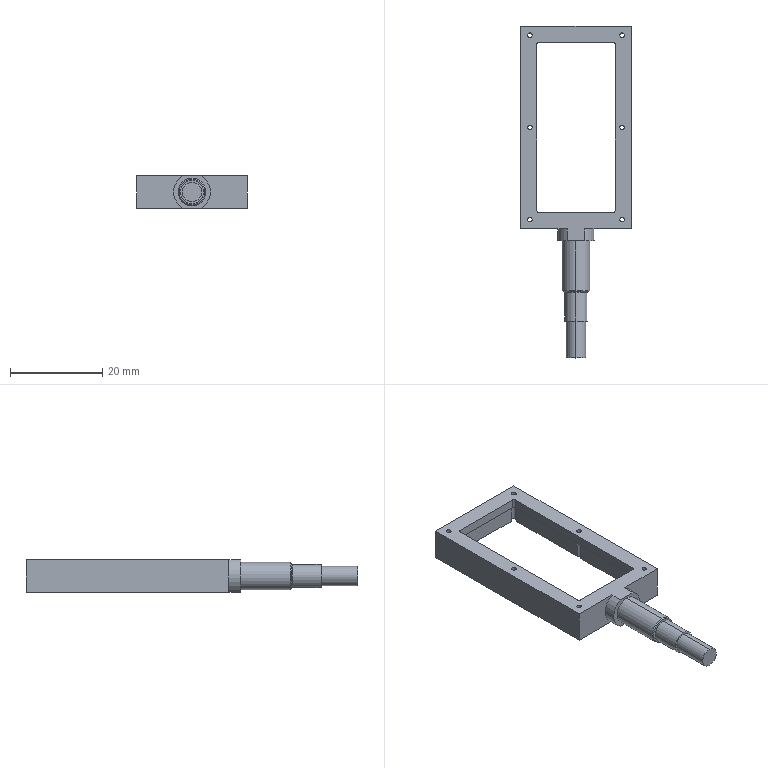NC program | NX | posted with a generic post | part box 24 x 72 x 7 mm
Lines 1 to 2080 of 5160, first 1994 of 2064 lines:
N10 G17 G21 G94 G90
(FLOOR_WALL , TOOL : D10)
N12 T10 M6
N14 G54
N16 G17 G0 G90 X-11.482 Y22. S9500 M3
N18 G43 Z30. H10
N20 Z2.505
N22 G94 G1 Z-0.495 F1000.
N24 X-3.482
N26 Y0. F2500.
N28 X3.482
N30 Y44.
N32 X-3.482
N34 Y22.
N36 X-11.482
N38 Z2.505
N40 G0 Z30.
N42 X-12.873
N44 Z2.011
N46 G1 Z-0.989 F1000.
N48 X0.373
N50 Y39.5 F2500.
N52 X-0.373
N54 Y4.5
N56 X0.373
N58 Y22.
N60 X4.873
N62 Y44.
N64 X-4.873
N66 Y0.
N68 X4.873
N70 Y22.
N72 X12.873
N74 Z2.011
N76 G0 Z30.
N78 X13.907
N80 Z1.516
N82 G1 Z-1.484 F1000.
N84 X0.907
N86 Y39. F2500.
N88 X-0.907
N90 Y5.
N92 X0.907
N94 Y22.
N96 X5.907
N98 Y44.
N100 X-5.907
N102 Y0.
N104 X5.907
N106 Y22.
N108 X13.907
N110 Z1.516
N112 G0 Z30.
N114 X14.748
N116 Z1.022
N118 G1 Z-1.978 F1000.
N120 X1.748
N122 Y39. F2500.
N124 X-1.748
N126 Y5.
N128 X1.748
N130 Y22.
N132 X6.748
N134 Y44.
N136 X-6.748
N138 Y0.
N140 X6.748
N142 Y22.
N144 X14.748
N146 Z1.022
N148 G0 Z30.
N150 X15.463
N152 Z0.528
N154 G1 Z-2.472 F1000.
N156 X2.463
N158 Y39. F2500.
N160 X-2.463
N162 Y5.
N164 X2.463
N166 Y22.
N168 X7.463
N170 Y44.
N172 X-7.463
N174 Y0.
N176 X7.463
N178 Y22.
N180 X15.463
N182 Z0.528
N184 G0 Z30.
N186 X16.085
N188 Z0.033
N190 G1 Z-2.967 F1000.
N192 X3.085
N194 Y39. F2500.
N196 X-3.085
N198 Y5.
N200 X3.085
N202 Y22.
N204 X8.085
N206 Y44.
N208 X-8.085
N210 Y0.
N212 X8.085
N214 Y22.
N216 X16.085
N218 Z0.033
N220 G0 Z30.
N222 X16.634
N224 Z-0.461
N226 G1 Z-3.461 F1000.
N228 X3.634
N230 Y39. F2500.
N232 X-3.634
N234 Y5.
N236 X3.634
N238 Y22.
N240 X8.634
N242 Y44.
N244 X-8.634
N246 Y0.
N248 X8.634
N250 Y22.
N252 X16.634
N254 Z-0.461
N256 G0 Z30.
N258 X17.124
N260 Z-0.956
N262 G1 Z-3.956 F1000.
N264 X4.124
N266 Y39. F2500.
N268 X-4.124
N270 Y5.
N272 X4.124
N274 Y22.
N276 X9.124
N278 Y44.
N280 X-9.124
N282 Y0.
N284 X9.124
N286 Y22.
N288 X17.124
N290 Z-0.956
N292 G0 Z30.
N294 X-0.063 Y9.915
N296 Z-0.956
N298 G1 Y9.5 Z-1.067 F1000.
N300 X0.063 Z-1.101
N302 Y22. Z-4.45
N304 Y34.5 F2500.
N306 X-0.063
N308 Y9.5
N310 X0.063
N312 Y22.
N314 X4.563
N316 Y39.
N318 X-4.563
N320 Y5.
N322 X4.563
N324 Y22.
N326 X9.563
N328 Y44.
N330 X-9.563
N332 Y0.
N334 X9.563
N336 Y22.
N338 X17.563
N340 Z-1.45
N342 G0 Z30.
N344 X-0.083 Y9.5
N346 Z-1.45
N348 G1 X0.458 Z-1.595 F1000.
N350 Y22. Z-4.945
N352 Y34.5 F2500.
N354 X-0.458
N356 Y9.5
N358 X0.458
N360 Y22.
N362 X4.958
N364 Y39.
N366 X-4.958
N368 Y5.
N370 X4.958
N372 Y22.
N374 X9.958
N376 Y44.
N378 X-9.958
N380 Y0.
N382 X9.958
N384 Y22.
N386 X17.958
N388 Z-1.945
N390 G0 Z30.
N392 X0.315 Y33.588
N394 Z-1.945
N396 G1 Y34. Z-2.055 F1000.
N398 X-0.315 Z-2.224
N400 Y22. Z-5.439
N402 Y10. F2500.
N404 X0.315
N406 Y34.
N408 X-0.315
N410 Y22.
N412 X-5.315
N414 Y5.
N416 X5.315
N418 Y39.
N420 X-5.315
N422 Y22.
N424 X-10.315
N426 Y0.
N428 X10.315
N430 Y44.
N432 X-10.315
N434 Y22.
N436 X-18.315
N438 Z-2.439
N440 G0 Z30.
N442 X0.405 Y34.
N444 Z-2.439
N446 G1 X-0.636 Z-2.718 F1000.
N448 Y22. Z-5.933
N450 Y10. F2500.
N452 X0.636
N454 Y34.
N456 X-0.636
N458 Y22.
N460 X-5.636
N462 Y5.
N464 X5.636
N466 Y39.
N468 X-5.636
N470 Y22.
N472 X-10.636
N474 Y0.
N476 X10.636
N478 Y44.
N480 X-10.636
N482 Y22.
N484 X-18.636
N486 Z-2.933
N488 G0 Z30.
N490 X-0.115 Y10.
N492 Z-2.933
N494 G1 X0.926 Z-3.212 F1000.
N496 Y22. Z-6.428
N498 Y34. F2500.
N500 X-0.926
N502 Y10.
N504 X0.926
N506 Y22.
N508 X5.926
N510 Y39.
N512 X-5.926
N514 Y5.
N516 X5.926
N518 Y22.
N520 X10.926
N522 Y44.
N524 X-10.926
N526 Y0.
N528 X10.926
N530 Y22.
N532 X18.926
N534 Z-3.428
N536 G0 Z30.
N538 X-0.145 Y34.
N540 Z-3.428
N542 G1 X-1.187 Z-3.707 F1000.
N544 Y22. Z-6.922
N546 Y10. F2500.
N548 X1.187
N550 Y34.
N552 X-1.187
N554 Y22.
N556 X-6.187
N558 Y5.
N560 X6.187
N562 Y39.
N564 X-6.187
N566 Y22.
N568 X-11.187
N570 Y0.
N572 X11.187
N574 Y44.
N576 X-11.187
N578 Y22.
N580 X-19.187
N582 Z-3.922
N584 G0 Z30.
N586 X-0.378 Y34.
N588 Z-3.922
N590 G1 X-1.42 Z-4.201 F1000.
N592 Y22. Z-7.417
N594 Y10. F2500.
N596 X1.42
N598 Y34.
N600 X-1.42
N602 Y22.
N604 X-6.42
N606 Y5.
N608 X6.42
N610 Y39.
N612 X-6.42
N614 Y22.
N616 X-11.42
N618 Y0.
N620 X11.42
N622 Y44.
N624 X-11.42
N626 Y22.
N628 X-19.42
N630 Z-4.417
N632 G0 Z30.
N634 X0.586 Y10.
N636 Z-4.417
N638 G1 X1.627 Z-4.696 F1000.
N640 Y22. Z-7.911
N642 Y34. F2500.
N644 X-1.627
N646 Y10.
N648 X1.627
N650 Y22.
N652 X6.627
N654 Y39.
N656 X-6.627
N658 Y5.
N660 X6.627
N662 Y22.
N664 X11.627
N666 Y44.
N668 X-11.627
N670 Y0.
N672 X11.627
N674 Y22.
N676 X19.627
N678 Z-4.911
N680 G0 Z30.
N682 X0.769 Y10.
N684 Z-4.911
N686 G1 X1.81 Z-5.19 F1000.
N688 Y22. Z-8.406
N690 Y34. F2500.
N692 X-1.81
N694 Y10.
N696 X1.81
N698 Y22.
N700 X6.81
N702 Y39.
N704 X-6.81
N706 Y5.
N708 X6.81
N710 Y22.
N712 X11.81
N714 Y44.
N716 X-11.81
N718 Y0.
N720 X11.81
N722 Y22.
N724 X19.81
N726 Z-5.406
N728 G0 Z30.
N730 X-0.929 Y34.003
N732 Z-5.406
N734 G1 X-1.97 Y34. Z-5.685 F1000.
N736 Y22. Z-8.9
N738 Y10. F2500.
N740 X1.97
N742 Y34.
N744 X1.744
N746 G2 X0. Y34.153 R10.
N748 X-1.744 Y34. R10.
N750 G1 X-1.97
N752 Y22.
N754 X-6.97
N756 Y5.
N758 X6.97
N760 Y39.
N762 X1.744
N764 G2 X0. Y39.314 R5.
N766 X-1.744 Y39. R5.
N768 G1 X-6.97
N770 Y22.
N772 X-11.97
N774 Y0.
N776 X11.97
N778 Y44.
N780 X1.744
N782 Y46.6
N784 X-1.744
N786 Y44.
N788 X-11.97
N790 Y22.
N792 X-19.97
N794 Z-5.9
N796 G0 Z30.
N798 M5
(DRILLING_COPY_1 , TOOL : D6A45)
N800 T07 M6
N802 G54
N804 G17 G0 G90 X-10. Y2. S5000 M3
N806 G43 Z30. H7
N808 G94 G81 G98 Z-10. F250. R-6.
N810 X-11. Y9.
N812 X-10. Y22.
N814 X-11. Y35.
N816 X-10. Y42.
N818 X10.
N820 X11. Y35.
N822 X10. Y22.
N824 X11. Y9.
N826 X10. Y2.
N828 G80
N830 G0 X10. Y2. Z30.
N832 M5
(DRILLING_COPY , TOOL : 1.25ZT)
N834 T14 M6
N836 G54
N838 G17 G0 G90 X11. Y35. S2009 M3
N840 G43 Z30. H14
N842 G94 G83 G98 Z-13.626 F100. Q2. R-6.
N844 X-11.
N846 Y9.
N848 X11.
N850 G80
N852 G0 X11. Y9. Z30.
N854 M5
(DRILLING_COPY_COPY , TOOL : 1.0ZT)
N856 T13 M6
N858 G54
N860 G17 G0 G90 X-10. Y22. S2009 M3
N862 G43 Z30. H13
N864 G94 G83 G98 Z-16.8 F100. Q2. R-6.
N866 Y2.
N868 X10.
N870 Y22.
N872 Y42.
N874 X-10.
N876 G80
N878 G0 X-10. Y42. Z30.
N880 M5
(CAVITY_MILL , TOOL : D10)
N882 T10 M6
N884 G54
N886 G17 G0 G90 X-19.132 Y24.145 S9500 M3
N888 G43 Z30. H10
N890 Z-8.49
N892 G94 G1 Z-9.49 F1000.
N894 X-17.489 Y22.766
N896 G2 X-17.132 Y22. R1.
N898 G1 Y0. F2500.
N900 G3 X-17. Y-1.143 R4.999
N902 G1 Y-1.005
N904 G2 X-17.1 Y0. R5.1
N906 G1 Y44.
N908 G2 X-17. Y45.005 R5.1
N910 G1 Y45.143
N912 G3 X-17.132 Y44. R4.999
N914 G1 Y22.
N916 G2 X-17.489 Y21.234 R1.
N918 G1 X-19.132 Y19.855
N920 Z-8.49
N922 G0 X-19.243 Y24.145 Z-8.98
N924 G1 Z-9.98 F1000.
N926 X-17.601 Y22.766
N928 G2 X-17.243 Y22. R1.
N930 G1 X-17.1
N932 Y44. F2500.
N934 G2 X-17. Y45.005 R5.1
N936 G1 Y45.541
N938 G3 X-17.243 Y44. R4.999
N940 G1 Y0.
N942 G3 X-17. Y-1.541 R4.999
N944 G1 Y-1.005
N946 G2 X-17.1 Y0. R5.1
N948 G1 Y22.
N950 G3 X-17.457 Y22.766 R1.
N952 G1 X-19.243 Y24.265
N954 Z-8.98
N956 G0 X-19.334 Y24.145 Z-9.47
N958 G1 Z-10.47 F1000.
N960 X-17.691 Y22.766
N962 G2 X-17.334 Y22. R1.
N964 G1 X-17.1
N966 Y44. F2500.
N968 G2 X-17. Y45.005 R5.1
N970 G1 Y45.797
N972 G3 X-17.334 Y44. R5.
N974 G1 Y0.
N976 G3 X-17. Y-1.797 R5.
N978 G1 Y-1.005
N980 G2 X-17.1 Y0. R5.1
N982 G1 Y22.
N984 G3 X-17.457 Y22.766 R1.
N986 G1 X-19.334 Y24.341
N988 Z-9.47
N990 G0 X-19.405 Y24.145 Z-9.96
N992 G1 Z-10.96 F1000.
N994 X-17.762 Y22.766
N996 G2 X-17.405 Y22. R1.
N998 G1 X-17.1
N1000 Y44. F2500.
N1002 G2 X-17. Y45.005 R5.1
N1004 G1 Y45.955
N1006 G3 X-17.405 Y44. R5.021
N1008 G1 Y0.
N1010 G3 X-17. Y-1.971 R5.
N1012 G1 Y-1.005
N1014 G2 X-17.1 Y0. R5.1
N1016 G1 Y22.
N1018 G3 X-17.457 Y22.766 R1.
N1020 G1 X-19.405 Y24.4
N1022 Z-9.96
N1024 G0 X-19.456 Y24.145 Z-10.45
N1026 G1 Z-11.45 F1000.
N1028 X-17.813 Y22.766
N1030 G2 X-17.456 Y22. R1.
N1032 G1 X-17.1
N1034 Y44. F2500.
N1036 G2 X-17. Y45.005 R5.1
N1038 G1 Y46.065
N1040 G3 X-17.456 Y44. R5.028
N1042 G1 Y0.
N1044 G3 X-17. Y-2.065 R5.027
N1046 G1 Y-1.005
N1048 G2 X-17.1 Y0. R5.1
N1050 G1 Y22.
N1052 G3 X-17.457 Y22.766 R1.
N1054 G1 X-19.456 Y24.443
N1056 Z-10.45
N1058 G0 X-19.487 Y24.145 Z-10.94
N1060 G1 Z-11.94 F1000.
N1062 X-17.845 Y22.766
N1064 G2 X-17.487 Y22. R1.
N1066 G1 X-17.1
N1068 Y44. F2500.
N1070 G2 X-17. Y45.005 R5.1
N1072 G1 Y46.14
N1074 G3 X-17.487 Y44. R5.018
N1076 G1 Y0.034
N1078 G3 X-17. Y-2.14 R5.017
N1080 G1 Y-1.005
N1082 G2 X-17.1 Y0. R5.1
N1084 G1 Y22.
N1086 G3 X-17.457 Y22.766 R1.
N1088 G1 X-19.487 Y24.47
N1090 Z-10.94
N1092 G0 X-19.5 Y24.145 Z-11.43
N1094 G1 Z-12.43 F1000.
N1096 X-17.857 Y22.766
N1098 G2 X-17.5 Y22. R1.
N1100 G1 X-17.1
N1102 Y44. F2500.
N1104 G2 X-17. Y45.005 R5.1
N1106 G1 Y46.179
N1108 G3 X-17.5 Y44. R5.001
N1110 G1 Y0.
N1112 G3 X-17. Y-2.176 R5.004
N1114 G1 Y-1.005
N1116 G2 X-17.1 Y0. R5.1
N1118 G1 Y22.
N1120 G3 X-17.457 Y22.766 R1.
N1122 G1 X-19.5 Y24.48
N1124 Z-11.43
N1126 G0 Y24.144 Z-11.92
N1128 G1 Z-12.92 F1000.
N1130 X-17.857 Y22.766
N1132 G2 X-17.5 Y22. R1.
N1134 G1 X-17.35
N1136 X-17.1
N1138 Y44. F2500.
N1140 G2 X-17. Y45.005 R5.1
N1142 G1 Y46.179
N1144 G3 X-17.5 Y44.011 R5.
N1146 G1 X-17.499 Y0.
N1148 G3 X-17. Y-2.173 R5.007
N1150 G1 Y-1.005
N1152 G2 X-17.1 Y0. R5.1
N1154 G1 Y22.
N1156 G3 X-17.457 Y22.766 R1.
N1158 G1 X-19.5 Y24.48
N1160 Z-11.92
N1162 G0 Y24.144 Z-12.41
N1164 G1 Z-13.41 F1000.
N1166 X-17.857 Y22.766
N1168 G2 X-17.5 Y22. R1.
N1170 G1 X-17.35
N1172 X-17.1
N1174 Y44. F2500.
N1176 G2 X-17. Y45.005 R5.1
N1178 G1 Y46.179
N1180 G3 X-17.5 Y44.011 R5.
N1182 G1 X-17.499 Y0.
N1184 G3 X-17. Y-2.173 R5.007
N1186 G1 Y-1.005
N1188 G2 X-17.1 Y0. R5.1
N1190 G1 Y22.
N1192 G3 X-17.457 Y22.766 R1.
N1194 G1 X-19.5 Y24.48
N1196 Z-12.41
N1198 G0 Y24.144 Z-12.9
N1200 G1 Z-13.9 F1000.
N1202 X-17.857 Y22.766
N1204 G2 X-17.5 Y22. R1.
N1206 G1 X-17.35
N1208 X-17.1
N1210 Y44. F2500.
N1212 G2 X-17. Y45.005 R5.1
N1214 G1 Y46.179
N1216 G3 X-17.5 Y44.011 R5.
N1218 G1 X-17.499 Y0.
N1220 G3 X-17. Y-2.173 R5.007
N1222 G1 Y-1.005
N1224 G2 X-17.1 Y0. R5.1
N1226 G1 Y22.
N1228 G3 X-17.457 Y22.766 R1.
N1230 G1 X-19.5 Y24.48
N1232 Z-12.9
N1234 G0 Y24.144 Z-13.32
N1236 G1 Z-14.32 F1000.
N1238 X-17.857 Y22.766
N1240 G2 X-17.5 Y22. R1.
N1242 G1 X-17.35
N1244 X-17.1
N1246 Y44. F2500.
N1248 G2 X-17. Y45.005 R5.1
N1250 G1 Y46.179
N1252 G3 X-17.5 Y44.011 R5.
N1254 G1 X-17.499 Y0.
N1256 G3 X-17. Y-2.173 R5.007
N1258 G1 Y-1.005
N1260 G2 X-17.1 Y0. R5.1
N1262 G1 Y22.
N1264 G3 X-17.457 Y22.766 R1.
N1266 G1 X-19.5 Y24.48
N1268 Z-13.32
N1270 G0 Y24.144 Z-13.74
N1272 G1 Z-14.74 F1000.
N1274 X-17.857 Y22.766
N1276 G2 X-17.5 Y22. R1.
N1278 G1 X-17.35
N1280 X-17.1
N1282 Y44. F2500.
N1284 G2 X-17. Y45.005 R5.1
N1286 G1 Y46.179
N1288 G3 X-17.5 Y44.011 R5.
N1290 G1 X-17.499 Y0.
N1292 G3 X-17. Y-2.173 R5.007
N1294 G1 Y-1.005
N1296 G2 X-17.1 Y0. R5.1
N1298 G1 Y22.
N1300 G3 X-17.457 Y22.766 R1.
N1302 G1 X-19.5 Y24.48
N1304 Z-13.74
N1306 G0 Y24.144 Z-14.16
N1308 G1 Z-15.16 F1000.
N1310 X-17.857 Y22.766
N1312 G2 X-17.5 Y22. R1.
N1314 G1 X-17.35
N1316 X-17.1
N1318 Y44. F2500.
N1320 G2 X-17. Y45.005 R5.1
N1322 G1 Y46.179
N1324 G3 X-17.5 Y44.011 R5.
N1326 G1 Y0.005
N1328 G3 X-17. Y-2.173 R5.008
N1330 G1 Y-1.005
N1332 G2 X-17.1 Y0. R5.1
N1334 G1 Y22.
N1336 G3 X-17.457 Y22.766 R1.
N1338 G1 X-19.5 Y24.48
N1340 Z-14.16
N1342 G0 Y24.144 Z-14.58
N1344 G1 Z-15.58 F1000.
N1346 X-17.857 Y22.766
N1348 G2 X-17.5 Y22. R1.
N1350 G1 X-17.35
N1352 X-17.1
N1354 Y44. F2500.
N1356 G2 X-17. Y45.005 R5.1
N1358 G1 Y46.179
N1360 G3 X-17.5 Y44.011 R5.
N1362 G1 Y0.005
N1364 G3 X-17. Y-2.173 R5.008
N1366 G1 Y-1.005
N1368 G2 X-17.1 Y0. R5.1
N1370 G1 Y22.
N1372 G3 X-17.457 Y22.766 R1.
N1374 G1 X-19.5 Y24.48
N1376 Z-14.58
N1378 G0 Y24.144 Z-15.
N1380 G1 Z-16. F1000.
N1382 X-17.857 Y22.766
N1384 G2 X-17.5 Y22. R1.
N1386 G1 X-17.35
N1388 X-17.1
N1390 Y44. F2500.
N1392 G2 X-17. Y45.005 R5.1
N1394 G1 Y46.179
N1396 G3 X-17.5 Y44.011 R5.
N1398 G1 Y0.005
N1400 G3 X-17. Y-2.173 R5.008
N1402 G1 Y-1.005
N1404 G2 X-17.1 Y0. R5.1
N1406 G1 Y22.
N1408 G3 X-17.457 Y22.766 R1.
N1410 G1 X-19.5 Y24.48
N1412 Z-15.
N1414 G0 Z30.
N1416 X-0.4 Y16.77
N1418 Z-7.5
N1420 G1 Y11.6 Z-7.771 F1000.
N1422 X0.4 Z-7.813
N1424 Y21.75 Z-8.345
N1426 X0.413 Y22. Z-8.358
N1428 X0.4 Y22.25 Z-8.371
N1430 Y32.4 Z-8.903
N1432 X-0.4 Z-8.945
N1434 Y22.25 Z-9.477
N1436 X-0.413 Y22. Z-9.49
N1438 G2 X-0.4 Y21.5 R9.6 F2500.
N1440 G1 Y11.6
N1442 X0.4
N1444 Y21.5
N1446 G2 X0.413 Y22. R9.6
N1448 X0.4 Y22.5 R9.6
N1450 G1 Y32.4
N1452 X-0.4
N1454 Y22.5
N1456 G2 X-0.413 Y22. R9.6
N1458 G1 X-4.907 Y22.234
N1460 G2 X-4.925 Y22. R5.1
N1462 X-4.9 Y21.5 R5.1
N1464 G1 Y7.1
N1466 X4.9
N1468 Y21.5
N1470 G2 X4.925 Y22. R5.1
N1472 X4.9 Y22.5 R5.1
N1474 G1 Y36.9
N1476 X-4.9
N1478 Y22.5
N1480 G2 X-4.907 Y22.234 R5.1
N1482 G3 X-4.59 Y21.451 R1.
N1484 G1 Z-8.49
N1486 G0 Z30.
N1488 X-0.4 Y16.77
N1490 Z-7.99
N1492 G1 Y11.6 Z-8.261 F1000.
N1494 X0.4 Z-8.303
N1496 Y21.75 Z-8.835
N1498 X0.413 Y22. Z-8.848
N1500 X0.4 Y22.25 Z-8.861
N1502 Y32.4 Z-9.393
N1504 X-0.4 Z-9.435
N1506 Y22.25 Z-9.967
N1508 X-0.413 Y22. Z-9.98
N1510 G2 X-0.4 Y21.5 R9.6 F2500.
N1512 G1 Y11.6
N1514 X0.4
N1516 Y21.5
N1518 G2 X0.413 Y22. R9.6
N1520 X0.4 Y22.5 R9.6
N1522 G1 Y32.4
N1524 X-0.4
N1526 Y22.5
N1528 G2 X-0.413 Y22. R9.6
N1530 G1 X-4.907 Y22.234
N1532 G2 X-4.925 Y22. R5.1
N1534 X-4.9 Y21.5 R5.1
N1536 G1 Y7.1
N1538 X4.9
N1540 Y21.5
N1542 G2 X4.925 Y22. R5.1
N1544 X4.9 Y22.5 R5.1
N1546 G1 Y36.9
N1548 X-4.9
N1550 Y22.5
N1552 G2 X-4.907 Y22.234 R5.1
N1554 G3 X-4.59 Y21.451 R1.
N1556 G1 Z-8.98
N1558 G0 Z30.
N1560 X-0.4 Y16.77
N1562 Z-8.48
N1564 G1 Y11.6 Z-8.751 F1000.
N1566 X0.4 Z-8.793
N1568 Y21.75 Z-9.325
N1570 X0.413 Y22. Z-9.338
N1572 X0.4 Y22.25 Z-9.351
N1574 Y32.4 Z-9.883
N1576 X-0.4 Z-9.925
N1578 Y22.25 Z-10.457
N1580 X-0.413 Y22. Z-10.47
N1582 G2 X-0.4 Y21.5 R9.6 F2500.
N1584 G1 Y11.6
N1586 X0.4
N1588 Y21.5
N1590 G2 X0.413 Y22. R9.6
N1592 X0.4 Y22.5 R9.6
N1594 G1 Y32.4
N1596 X-0.4
N1598 Y22.5
N1600 G2 X-0.413 Y22. R9.6
N1602 G1 X-4.907 Y22.234
N1604 G2 X-4.925 Y22. R5.1
N1606 X-4.9 Y21.5 R5.1
N1608 G1 Y7.1
N1610 X4.9
N1612 Y21.5
N1614 G2 X4.925 Y22. R5.1
N1616 X4.9 Y22.5 R5.1
N1618 G1 Y36.9
N1620 X-4.9
N1622 Y22.5
N1624 G2 X-4.907 Y22.234 R5.1
N1626 G3 X-4.59 Y21.451 R1.
N1628 G1 Z-9.47
N1630 G0 X-0.4 Y16.77 Z-8.97
N1632 G1 Y11.6 Z-9.241 F1000.
N1634 X0.4 Z-9.283
N1636 Y21.75 Z-9.815
N1638 X0.413 Y22. Z-9.828
N1640 X0.4 Y22.25 Z-9.841
N1642 Y32.4 Z-10.373
N1644 X-0.4 Z-10.415
N1646 Y22.25 Z-10.947
N1648 X-0.413 Y22. Z-10.96
N1650 G2 X-0.4 Y21.5 R9.6 F2500.
N1652 G1 Y11.6
N1654 X0.4
N1656 Y21.5
N1658 G2 X0.413 Y22. R9.6
N1660 X0.4 Y22.5 R9.6
N1662 G1 Y32.4
N1664 X-0.4
N1666 Y22.5
N1668 G2 X-0.413 Y22. R9.6
N1670 G1 X-4.907 Y22.234
N1672 G2 X-4.925 Y22. R5.1
N1674 X-4.9 Y21.5 R5.1
N1676 G1 Y7.1
N1678 X4.9
N1680 Y21.5
N1682 G2 X4.925 Y22. R5.1
N1684 X4.9 Y22.5 R5.1
N1686 G1 Y36.9
N1688 X-4.9
N1690 Y22.5
N1692 G2 X-4.907 Y22.234 R5.1
N1694 G3 X-4.59 Y21.451 R1.
N1696 G1 Z-9.96
N1698 G0 X-0.4 Y16.77 Z-9.46
N1700 G1 Y11.6 Z-9.731 F1000.
N1702 X0.4 Z-9.773
N1704 Y21.75 Z-10.305
N1706 X0.413 Y22. Z-10.318
N1708 X0.4 Y22.25 Z-10.331
N1710 Y32.4 Z-10.863
N1712 X-0.4 Z-10.905
N1714 Y22.25 Z-11.437
N1716 X-0.413 Y22. Z-11.45
N1718 G2 X-0.4 Y21.5 R9.6 F2500.
N1720 G1 Y11.6
N1722 X0.4
N1724 Y21.5
N1726 G2 X0.413 Y22. R9.6
N1728 X0.4 Y22.5 R9.6
N1730 G1 Y32.4
N1732 X-0.4
N1734 Y22.5
N1736 G2 X-0.413 Y22. R9.6
N1738 G1 X-4.907 Y22.234
N1740 G2 X-4.925 Y22. R5.1
N1742 X-4.9 Y21.5 R5.1
N1744 G1 Y7.1
N1746 X4.9
N1748 Y21.5
N1750 G2 X4.925 Y22. R5.1
N1752 X4.9 Y22.5 R5.1
N1754 G1 Y36.9
N1756 X-4.9
N1758 Y22.5
N1760 G2 X-4.907 Y22.234 R5.1
N1762 G3 X-4.59 Y21.451 R1.
N1764 G1 Z-10.45
N1766 G0 X-0.4 Y16.77 Z-9.95
N1768 G1 Y11.6 Z-10.221 F1000.
N1770 X0.4 Z-10.263
N1772 Y21.75 Z-10.795
N1774 X0.413 Y22. Z-10.808
N1776 X0.4 Y22.25 Z-10.821
N1778 Y32.4 Z-11.353
N1780 X-0.4 Z-11.395
N1782 Y22.25 Z-11.927
N1784 X-0.413 Y22. Z-11.94
N1786 G2 X-0.4 Y21.5 R9.6 F2500.
N1788 G1 Y11.6
N1790 X0.4
N1792 Y21.5
N1794 G2 X0.413 Y22. R9.6
N1796 X0.4 Y22.5 R9.6
N1798 G1 Y32.4
N1800 X-0.4
N1802 Y22.5
N1804 G2 X-0.413 Y22. R9.6
N1806 G1 X-4.907 Y22.234
N1808 G2 X-4.925 Y22. R5.1
N1810 X-4.9 Y21.5 R5.1
N1812 G1 Y7.1
N1814 X4.9
N1816 Y21.5
N1818 G2 X4.925 Y22. R5.1
N1820 X4.9 Y22.5 R5.1
N1822 G1 Y36.9
N1824 X-4.9
N1826 Y22.5
N1828 G2 X-4.907 Y22.234 R5.1
N1830 G3 X-4.59 Y21.451 R1.
N1832 G1 Z-10.94
N1834 G0 X-0.4 Y16.77 Z-10.44
N1836 G1 Y11.6 Z-10.711 F1000.
N1838 X0.4 Z-10.753
N1840 Y21.75 Z-11.285
N1842 X0.413 Y22. Z-11.298
N1844 X0.4 Y22.25 Z-11.311
N1846 Y32.4 Z-11.843
N1848 X-0.4 Z-11.885
N1850 Y22.25 Z-12.417
N1852 X-0.413 Y22. Z-12.43
N1854 G2 X-0.4 Y21.5 R9.6 F2500.
N1856 G1 Y11.6
N1858 X0.4
N1860 Y21.5
N1862 G2 X0.413 Y22. R9.6
N1864 X0.4 Y22.5 R9.6
N1866 G1 Y32.4
N1868 X-0.4
N1870 Y22.5
N1872 G2 X-0.413 Y22. R9.6
N1874 G1 X-4.907 Y22.234
N1876 G2 X-4.925 Y22. R5.1
N1878 X-4.9 Y21.5 R5.1
N1880 G1 Y7.1
N1882 X4.9
N1884 Y21.5
N1886 G2 X4.925 Y22. R5.1
N1888 X4.9 Y22.5 R5.1
N1890 G1 Y36.9
N1892 X-4.9
N1894 Y22.5
N1896 G2 X-4.907 Y22.234 R5.1
N1898 G3 X-4.59 Y21.451 R1.
N1900 G1 Z-11.43
N1902 G0 X-0.4 Y16.77 Z-10.93
N1904 G1 Y11.6 Z-11.201 F1000.
N1906 X0.4 Z-11.243
N1908 Y21.75 Z-11.775
N1910 X0.413 Y22. Z-11.788
N1912 X0.4 Y22.25 Z-11.801
N1914 Y32.4 Z-12.333
N1916 X-0.4 Z-12.375
N1918 Y22.25 Z-12.907
N1920 X-0.413 Y22. Z-12.92
N1922 G2 X-0.4 Y21.5 R9.6 F2500.
N1924 G1 Y11.6
N1926 X0.4
N1928 Y21.5
N1930 G2 X0.413 Y22. R9.6
N1932 X0.4 Y22.5 R9.6
N1934 G1 Y32.4
N1936 X-0.4
N1938 Y22.5
N1940 G2 X-0.413 Y22. R9.6
N1942 G1 X-4.907 Y22.234
N1944 G2 X-4.925 Y22. R5.1
N1946 X-4.9 Y21.5 R5.1
N1948 G1 Y7.1
N1950 X4.9
N1952 Y21.5
N1954 G2 X4.925 Y22. R5.1
N1956 X4.9 Y22.5 R5.1
N1958 G1 Y36.9
N1960 X-4.9
N1962 Y22.5
N1964 G2 X-4.907 Y22.234 R5.1
N1966 G3 X-4.59 Y21.451 R1.
N1968 G1 Z-11.92
N1970 G0 X-0.4 Y16.77 Z-11.42
N1972 G1 Y11.6 Z-11.691 F1000.
N1974 X0.4 Z-11.733
N1976 Y21.75 Z-12.265
N1978 X0.413 Y22. Z-12.278
N1980 X0.4 Y22.25 Z-12.291
N1982 Y32.4 Z-12.823
N1984 X-0.4 Z-12.865
N1986 Y22.25 Z-13.397
N1988 X-0.413 Y22. Z-13.41
N1990 G2 X-0.4 Y21.5 R9.6 F2500.
N1992 G1 Y11.6
N1994 X0.4
N1996 Y21.5
N1998 G2 X0.413 Y22. R9.6
N2000 X0.4 Y22.5 R9.6
N2002 G1 Y32.4
N2004 X-0.4
N2006 Y22.5
N2008 G2 X-0.413 Y22. R9.6
N2010 G1 X-4.907 Y22.234
N2012 G2 X-4.925 Y22. R5.1
N2014 X-4.9 Y21.5 R5.1
N2016 G1 Y7.1
N2018 X4.9
N2020 Y21.5
N2022 G2 X4.925 Y22. R5.1
N2024 X4.9 Y22.5 R5.1
N2026 G1 Y36.9
N2028 X-4.9
N2030 Y22.5
N2032 G2 X-4.907 Y22.234 R5.1
N2034 G3 X-4.59 Y21.451 R1.
N2036 G1 Z-12.41
N2038 G0 X-0.4 Y16.77 Z-11.91
N2040 G1 Y11.6 Z-12.181 F1000.
N2042 X0.4 Z-12.223
N2044 Y21.75 Z-12.755
N2046 X0.413 Y22. Z-12.768
N2048 X0.4 Y22.25 Z-12.781
N2050 Y32.4 Z-13.313
N2052 X-0.4 Z-13.355
N2054 Y22.25 Z-13.887
N2056 X-0.413 Y22. Z-13.9
N2058 G2 X-0.4 Y21.5 R9.6 F2500.
N2060 G1 Y11.6
N2062 X0.4
N2064 Y21.5
N2066 G2 X0.413 Y22. R9.6
N2068 X0.4 Y22.5 R9.6
N2070 G1 Y32.4
N2072 X-0.4
N2074 Y22.5
N2076 G2 X-0.413 Y22. R9.6
N2078 G1 X-4.907 Y22.234
N2080 G2 X-4.925 Y22. R5.1
N2082 X-4.9 Y21.5 R5.1
N2084 G1 Y7.1
N2086 X4.9
N2088 Y21.5
N2090 G2 X4.925 Y22. R5.1
N2092 X4.9 Y22.5 R5.1
N2094 G1 Y36.9
N2096 X-4.9
N2098 Y22.5
N2100 G2 X-4.907 Y22.234 R5.1
N2102 G3 X-4.59 Y21.451 R1.
N2104 G1 Z-12.9
N2106 G0 X3.4 Y18.964 Z-12.4
N2108 G1 Y35.4 Z-13.261 F1000.
N2110 X-3.4 Z-13.618
N2112 Y22. Z-14.32
N2114 Y8.6 F2500.
N2116 X3.4
N2118 Y35.4
N2120 X-3.4
N2122 Y22.
N2124 G3 X-3.043 Y21.234 R1.
N2126 G1 Z-13.32
N2128 G0 X3.4 Y18.964 Z-12.82
N2130 G1 Y35.4 Z-13.681 F1000.
N2132 X-3.4 Z-14.038
N2134 Y22. Z-14.74
N2136 Y8.6 F2500.
N2138 X3.4
N2140 Y35.4
N2142 X-3.4
N2144 Y22.
N2146 G3 X-3.043 Y21.234 R1.
N2148 G1 Z-13.74
N2150 G0 X3.4 Y18.964 Z-13.24
N2152 G1 Y35.4 Z-14.101 F1000.
N2154 X-3.4 Z-14.458
N2156 Y22. Z-15.16
N2158 Y8.6 F2500.
N2160 X3.4
N2162 Y35.4
N2164 X-3.4
N2166 Y22.
N2168 G3 X-3.043 Y21.234 R1.
N2170 G1 Z-14.16
N2172 G0 X3.4 Y18.964 Z-13.66
N2174 G1 Y35.4 Z-14.521 F1000.
N2176 X-3.4 Z-14.878
N2178 Y22. Z-15.58
N2180 Y8.6 F2500.
N2182 X3.4
N2184 Y35.4
N2186 X-3.4
N2188 Y22.
N2190 G3 X-3.043 Y21.234 R1.
N2192 G1 Z-14.58
N2194 G0 X3.4 Y18.964 Z-14.08
N2196 G1 Y35.4 Z-14.941 F1000.
N2198 X-3.4 Z-15.298
N2200 Y22. Z-16.
N2202 Y8.6 F2500.
N2204 X3.4
N2206 Y35.4
N2208 X-3.4
N2210 Y22.
N2212 G3 X-3.043 Y21.234 R1.
N2214 G1 Z-15.
N2216 G0 Z30.
N2218 X19.132 Y19.855
N2220 Z-8.49
N2222 G1 Z-9.49 F1000.
N2224 X17.489 Y21.234
N2226 G2 X17.132 Y22. R1.
N2228 G1 Y44. F2500.
N2230 G3 X17. Y45.142 R5.
N2232 G1 Y45.005
N2234 G2 X17.1 Y44. R5.1
N2236 G1 Y0.
N2238 G2 X17. Y-1.005 R5.1
N2240 G1 Y-1.142
N2242 G3 X17.132 Y0. R5.
N2244 G1 Y22.
N2246 G2 X17.489 Y22.766 R1.
N2248 G1 X19.132 Y24.145
N2250 Z-8.49
N2252 G0 X19.243 Y19.855 Z-8.98
N2254 G1 Z-9.98 F1000.
N2256 X17.601 Y21.234
N2258 G2 X17.243 Y22. R1.
N2260 G1 X17.1
N2262 Y0. F2500.
N2264 G2 X17. Y-1.005 R5.1
N2266 G1 Y-1.531
N2268 G3 X17.243 Y0. R5.012
N2270 G1 Y44.
N2272 G3 X17. Y45.541 R5.
N2274 G1 Y45.005
N2276 G2 X17.1 Y44. R5.1
N2278 G1 Y22.
N2280 G3 X17.457 Y21.234 R1.
N2282 G1 X19.243 Y19.735
N2284 Z-8.98
N2286 G0 X19.334 Y19.855 Z-9.47
N2288 G1 Z-10.47 F1000.
N2290 X17.691 Y21.234
N2292 G2 X17.334 Y22. R1.
N2294 G1 X17.1
N2296 Y0. F2500.
N2298 G2 X17. Y-1.005 R5.1
N2300 G1 Y-1.779
N2302 G3 X17.334 Y0. R5.022
N2304 G1 Y44.
N2306 G3 X17. Y45.78 R5.02
N2308 G1 Y45.005
N2310 G2 X17.1 Y44. R5.1
N2312 G1 Y22.
N2314 G3 X17.457 Y21.234 R1.
N2316 G1 X19.334 Y19.659
N2318 Z-9.47
N2320 G0 X19.405 Y19.855 Z-9.96
N2322 G1 Z-10.96 F1000.
N2324 X17.762 Y21.234
N2326 G2 X17.405 Y22. R1.
N2328 G1 X17.1
N2330 Y0. F2500.
N2332 G2 X17. Y-1.005 R5.1
N2334 G1 Y-1.961
N2336 G3 X17.405 Y0. R5.013
N2338 G1 Y44.
N2340 G3 X17. Y45.971 R5.
N2342 G1 Y45.005
N2344 G2 X17.1 Y44. R5.1
N2346 G1 Y22.
N2348 G3 X17.457 Y21.234 R1.
N2350 G1 X19.405 Y19.6
N2352 Z-9.96
N2354 G0 X19.456 Y19.855 Z-10.45
N2356 G1 Z-11.45 F1000.
N2358 X17.813 Y21.234
N2360 G2 X17.456 Y22. R1.
N2362 G1 X17.1
N2364 Y0. F2500.
N2366 G2 X17. Y-1.005 R5.1
N2368 G1 Y-2.085
N2370 G3 X17.456 Y0. R5.001
N2372 G1 Y44.
N2374 G3 X17. Y46.065 R5.027
N2376 G1 Y45.005
N2378 G2 X17.1 Y44. R5.1
N2380 G1 Y22.
N2382 G3 X17.457 Y21.234 R1.
N2384 G1 X19.456 Y19.557
N2386 Z-10.45
N2388 G0 X19.487 Y19.855 Z-10.94
N2390 G1 Z-11.94 F1000.
N2392 X17.845 Y21.234
N2394 G2 X17.487 Y22. R1.
N2396 G1 X17.1
N2398 Y0. F2500.
N2400 G2 X17. Y-1.005 R5.1
N2402 G1 Y-2.133
N2404 G3 X17.487 Y0.051 R5.026
N2406 G1 Y44.
N2408 G3 X17. Y46.14 R5.018
N2410 G1 Y45.005
N2412 G2 X17.1 Y44. R5.1
N2414 G1 Y22.
N2416 G3 X17.457 Y21.234 R1.
N2418 G1 X19.487 Y19.53
N2420 Z-10.94
N2422 G0 X19.5 Y19.855 Z-11.43
N2424 G1 Z-12.43 F1000.
N2426 X17.857 Y21.234
N2428 G2 X17.5 Y22. R1.
N2430 G1 X17.1
N2432 Y0. F2500.
N2434 G2 X17. Y-1.005 R5.1
N2436 G1 Y-2.179
N2438 G3 X17.5 Y0. R5.001
N2440 G1 Y44.
N2442 G3 X17. Y46.174 R5.007
N2444 G1 Y45.005
N2446 G2 X17.1 Y44. R5.1
N2448 G1 Y22.
N2450 G3 X17.457 Y21.234 R1.
N2452 G1 X19.5 Y19.52
N2454 Z-11.43
N2456 G0 Y19.855 Z-11.92
N2458 G1 Z-12.92 F1000.
N2460 X17.857 Y21.234
N2462 G2 X17.5 Y22. R1.
N2464 G1 X17.35
N2466 X17.1
N2468 Y0. F2500.
N2470 G2 X17. Y-1.005 R5.1
N2472 G1 Y-2.173
N2474 G3 X17.499 Y0. R5.007
N2476 G1 X17.5 Y44.
N2478 G3 X17. Y46.177 R5.002
N2480 G1 Y45.005
N2482 G2 X17.1 Y44. R5.1
N2484 G1 Y22.
N2486 G3 X17.457 Y21.234 R1.
N2488 G1 X19.5 Y19.52
N2490 Z-11.92
N2492 G0 Y19.855 Z-12.41
N2494 G1 Z-13.41 F1000.
N2496 X17.857 Y21.234
N2498 G2 X17.5 Y22. R1.
N2500 G1 X17.35
N2502 X17.1
N2504 Y0. F2500.
N2506 G2 X17. Y-1.005 R5.1
N2508 G1 Y-2.173
N2510 G3 X17.499 Y0. R5.007
N2512 G1 X17.5 Y44.011
N2514 G3 X17. Y46.179 R5.
N2516 G1 Y45.005
N2518 G2 X17.1 Y44. R5.1
N2520 G1 Y22.
N2522 G3 X17.457 Y21.234 R1.
N2524 G1 X19.5 Y19.52
N2526 Z-12.41
N2528 G0 Y19.855 Z-12.9
N2530 G1 Z-13.9 F1000.
N2532 X17.857 Y21.234
N2534 G2 X17.5 Y22. R1.
N2536 G1 X17.35
N2538 X17.1
N2540 Y0. F2500.
N2542 G2 X17. Y-1.005 R5.1
N2544 G1 Y-2.173
N2546 G3 X17.499 Y0. R5.007
N2548 G1 X17.5 Y44.011
N2550 G3 X17. Y46.179 R5.
N2552 G1 Y45.005
N2554 G2 X17.1 Y44. R5.1
N2556 G1 Y22.
N2558 G3 X17.457 Y21.234 R1.
N2560 G1 X19.5 Y19.52
N2562 Z-12.9
N2564 G0 Y19.855 Z-13.32
N2566 G1 Z-14.32 F1000.
N2568 X17.857 Y21.234
N2570 G2 X17.5 Y22. R1.
N2572 G1 X17.35
N2574 X17.1
N2576 Y0. F2500.
N2578 G2 X17. Y-1.005 R5.1
N2580 G1 Y-2.173
N2582 G3 X17.499 Y0. R5.007
N2584 G1 X17.5 Y44.011
N2586 G3 X17. Y46.179 R5.
N2588 G1 Y45.005
N2590 G2 X17.1 Y44. R5.1
N2592 G1 Y22.
N2594 G3 X17.457 Y21.234 R1.
N2596 G1 X19.5 Y19.52
N2598 Z-13.32
N2600 G0 Y19.855 Z-13.74
N2602 G1 Z-14.74 F1000.
N2604 X17.857 Y21.234
N2606 G2 X17.5 Y22. R1.
N2608 G1 X17.35
N2610 X17.1
N2612 Y0. F2500.
N2614 G2 X17. Y-1.005 R5.1
N2616 G1 Y-2.173
N2618 G3 X17.499 Y0. R5.007
N2620 G1 X17.5 Y44.011
N2622 G3 X17. Y46.179 R5.
N2624 G1 Y45.005
N2626 G2 X17.1 Y44. R5.1
N2628 G1 Y22.
N2630 G3 X17.457 Y21.234 R1.
N2632 G1 X19.5 Y19.52
N2634 Z-13.74
N2636 G0 Y19.855 Z-14.16
N2638 G1 Z-15.16 F1000.
N2640 X17.857 Y21.234
N2642 G2 X17.5 Y22. R1.
N2644 G1 X17.35
N2646 X17.1
N2648 Y0. F2500.
N2650 G2 X17. Y-1.005 R5.1
N2652 G1 Y-2.173
N2654 G3 X17.5 Y0.005 R5.008
N2656 G1 Y44.011
N2658 G3 X17. Y46.179 R5.
N2660 G1 Y45.005
N2662 G2 X17.1 Y44. R5.1
N2664 G1 Y22.
N2666 G3 X17.457 Y21.234 R1.
N2668 G1 X19.5 Y19.52
N2670 Z-14.16
N2672 G0 Y19.855 Z-14.58
N2674 G1 Z-15.58 F1000.
N2676 X17.857 Y21.234
N2678 G2 X17.5 Y22. R1.
N2680 G1 X17.35
N2682 X17.1
N2684 Y0. F2500.
N2686 G2 X17. Y-1.005 R5.1
N2688 G1 Y-2.173
N2690 G3 X17.5 Y0.005 R5.008
N2692 G1 Y44.011
N2694 G3 X17. Y46.179 R5.
N2696 G1 Y45.005
N2698 G2 X17.1 Y44. R5.1
N2700 G1 Y22.
N2702 G3 X17.457 Y21.234 R1.
N2704 G1 X19.5 Y19.52
N2706 Z-14.58
N2708 G0 Y19.855 Z-15.
N2710 G1 Z-16. F1000.
N2712 X17.857 Y21.234
N2714 G2 X17.5 Y22. R1.
N2716 G1 X17.35
N2718 X17.1
N2720 Y0. F2500.
N2722 G2 X17. Y-1.005 R5.1
N2724 G1 Y-2.173
N2726 G3 X17.5 Y0.005 R5.008
N2728 G1 Y44.011
N2730 G3 X17. Y46.179 R5.
N2732 G1 Y45.005
N2734 G2 X17.1 Y44. R5.1
N2736 G1 Y22.
N2738 G3 X17.457 Y21.234 R1.
N2740 G1 X19.5 Y19.52
N2742 Z-15.
N2744 G0 Z30.
N2746 M5
(CAVITY_MILL_COPY , TOOL : D4)
N2748 T04 M6
N2750 G54
N2752 G17 G0 G90 X-3.965 Y39.2 S9504 M3
N2754 G43 Z30. H4
N2756 Z-8.385
N2758 G94 G1 Z-9.385 F1000.
N2760 X-4.337 Y39.643
N2762 G3 X-5.103 Y40. R1.
N2764 G1 X-8. F1650.
N2766 Y37.103
N2768 G3 X-7.643 Y36.337 R1.
N2770 G1 X-7.2 Y35.965
N2772 Z-8.385
N2774 G0 Z30.
N2776 X-3.965 Y39.2
N2778 Z-8.769
N2780 G1 Z-9.769 F1000.
N2782 X-4.337 Y39.643
N2784 G3 X-5.103 Y40. R1.
N2786 G1 X-8. F1650.
N2788 Y37.103
N2790 G3 X-7.643 Y36.337 R1.
N2792 G1 X-7.2 Y35.965
N2794 Z-8.769
N2796 G0 X-3.965 Y39.2 Z-9.154
N2798 G1 Z-10.154 F1000.
N2800 X-4.337 Y39.643
N2802 G3 X-5.103 Y40. R1.
N2804 G1 X-8. F1650.
N2806 Y37.103
N2808 G3 X-7.643 Y36.337 R1.
N2810 G1 X-7.2 Y35.965
N2812 Z-9.154
N2814 G0 X-3.965 Y39.2 Z-9.538
N2816 G1 Z-10.538 F1000.
N2818 X-4.337 Y39.643
N2820 G3 X-5.103 Y40. R1.
N2822 G1 X-8. F1650.
N2824 Y37.103
N2826 G3 X-7.643 Y36.337 R1.
N2828 G1 X-7.2 Y35.965
N2830 Z-9.538
N2832 G0 X-3.965 Y39.2 Z-9.923
N2834 G1 Z-10.923 F1000.
N2836 X-4.337 Y39.643
N2838 G3 X-5.103 Y40. R1.
N2840 G1 X-8. Y39.999 F1650.
N2842 Y37.103
N2844 G3 X-7.643 Y36.337 R1.
N2846 G1 X-7.2 Y35.965
N2848 Z-9.923
N2850 G0 X-3.965 Y39.2 Z-10.308
N2852 G1 Z-11.308 F1000.
N2854 X-4.337 Y39.643
N2856 G3 X-5.103 Y40. R1.
N2858 G1 X-8. Y39.999 F1650.
N2860 Y37.103
N2862 G3 X-7.643 Y36.337 R1.
N2864 G1 X-7.2 Y35.965
N2866 Z-10.308
N2868 G0 X-3.965 Y39.2 Z-10.692
N2870 G1 Z-11.692 F1000.
N2872 X-4.337 Y39.643
N2874 G3 X-5.103 Y40. R1.
N2876 G1 X-8. Y39.999 F1650.
N2878 Y37.103
N2880 G3 X-7.643 Y36.337 R1.
N2882 G1 X-7.2 Y35.965
N2884 Z-10.692
N2886 G0 X-3.965 Y39.2 Z-11.077
N2888 G1 Z-12.077 F1000.
N2890 X-4.337 Y39.643
N2892 G3 X-5.103 Y40. R1.
N2894 G1 X-8. Y39.999 F1650.
N2896 Y37.103
N2898 G3 X-7.643 Y36.337 R1.
N2900 G1 X-7.2 Y35.965
N2902 Z-11.077
N2904 G0 X-3.965 Y39.2 Z-11.462
N2906 G1 Z-12.462 F1000.
N2908 X-4.337 Y39.643
N2910 G3 X-5.103 Y40. R1.
N2912 G1 X-8. Y39.999 F1650.
N2914 Y37.103
N2916 G3 X-7.643 Y36.337 R1.
N2918 G1 X-7.2 Y35.965
N2920 Z-11.462
N2922 G0 X-3.965 Y39.2 Z-11.846
N2924 G1 Z-12.846 F1000.
N2926 X-4.337 Y39.643
N2928 G3 X-5.103 Y40. R1.
N2930 G1 X-8. Y39.999 F1650.
N2932 Y37.103
N2934 G3 X-7.643 Y36.337 R1.
N2936 G1 X-7.2 Y35.965
N2938 Z-11.846
N2940 G0 X-3.965 Y39.2 Z-12.231
N2942 G1 Z-13.231 F1000.
N2944 X-4.337 Y39.643
N2946 G3 X-5.103 Y40. R1.
N2948 G1 X-8. Y39.999 F1650.
N2950 Y37.103
N2952 G3 X-7.643 Y36.337 R1.
N2954 G1 X-7.2 Y35.965
N2956 Z-12.231
N2958 G0 X-3.965 Y39.2 Z-12.615
N2960 G1 Z-13.615 F1000.
N2962 X-4.337 Y39.643
N2964 G3 X-5.103 Y40. R1.
N2966 G1 X-8. Y39.999 F1650.
N2968 Y37.103
N2970 G3 X-7.643 Y36.337 R1.
N2972 G1 X-7.2 Y35.965
N2974 Z-12.615
N2976 G0 X-3.965 Y39.2 Z-13.
N2978 G1 Z-14. F1000.
N2980 X-4.337 Y39.643
N2982 G3 X-5.103 Y40. R1.
N2984 G1 X-8. Y39.998 F1650.
N2986 Y37.103
N2988 G3 X-7.643 Y36.337 R1.
N2990 G1 X-7.2 Y35.965
N2992 Z-13.
N2994 G0 X-2.465 Y37.7 Z-13.4
N2996 G1 Z-14.4 F1000.
N2998 X-2.837 Y38.143
N3000 G3 X-3.603 Y38.5 R1.
N3002 G1 X-6.5 F1650.
N3004 Y35.603
N3006 G3 X-6.143 Y34.837 R1.
N3008 G1 X-5.7 Y34.465
N3010 Z-13.4
N3012 G0 X-2.465 Y37.7 Z-13.8
N3014 G1 Z-14.8 F1000.
N3016 X-2.837 Y38.143
N3018 G3 X-3.603 Y38.5 R1.
N3020 G1 X-6.5 F1650.
N3022 Y35.603
N3024 G3 X-6.143 Y34.837 R1.
N3026 G1 X-5.7 Y34.465
N3028 Z-13.8
N3030 G0 X-2.465 Y37.7 Z-14.2
N3032 G1 Z-15.2 F1000.
N3034 X-2.837 Y38.143
N3036 G3 X-3.603 Y38.5 R1.
N3038 G1 X-6.5 F1650.
N3040 Y35.603
N3042 G3 X-6.143 Y34.837 R1.
N3044 G1 X-5.7 Y34.465
N3046 Z-14.2
N3048 G0 X-2.465 Y37.7 Z-14.6
N3050 G1 Z-15.6 F1000.
N3052 X-2.837 Y38.143
N3054 G3 X-3.603 Y38.5 R1.
N3056 G1 X-6.5 F1650.
N3058 Y35.603
N3060 G3 X-6.143 Y34.837 R1.
N3062 G1 X-5.7 Y34.465
N3064 Z-14.6
N3066 G0 X-2.465 Y37.7 Z-15.
N3068 G1 Z-16. F1000.
N3070 X-2.837 Y38.143
N3072 G3 X-3.603 Y38.5 R1.
N3074 G1 X-6.5 F1650.
N3076 Y35.603
N3078 G3 X-6.143 Y34.837 R1.
N3080 G1 X-5.7 Y34.465
N3082 Z-15.
N3084 G0 Z30.
N3086 X7.2 Y35.965
N3088 Z-8.385
N3090 G1 Z-9.385 F1000.
N3092 X7.643 Y36.337
N3094 G3 X8. Y37.103 R1.
N3096 G1 Y40. F1650.
N3098 X5.103
N3100 G3 X4.337 Y39.643 R1.
N3102 G1 X3.965 Y39.2
N3104 Z-8.385
N3106 G0 Z30.
N3108 X7.2 Y35.965
N3110 Z-8.769
N3112 G1 Z-9.769 F1000.
N3114 X7.643 Y36.337
N3116 G3 X8. Y37.103 R1.
N3118 G1 Y40. F1650.
N3120 X5.103
N3122 G3 X4.337 Y39.643 R1.
N3124 G1 X3.965 Y39.2
N3126 Z-8.769
N3128 G0 X7.2 Y35.965 Z-9.154
N3130 G1 Z-10.154 F1000.
N3132 X7.643 Y36.337
N3134 G3 X8. Y37.103 R1.
N3136 G1 Y40. F1650.
N3138 X5.103
N3140 G3 X4.337 Y39.643 R1.
N3142 G1 X3.965 Y39.2
N3144 Z-9.154
N3146 G0 X7.2 Y35.965 Z-9.538
N3148 G1 Z-10.538 F1000.
N3150 X7.643 Y36.337
N3152 G3 X8. Y37.103 R1.
N3154 G1 Y40. F1650.
N3156 X5.103
N3158 G3 X4.337 Y39.643 R1.
N3160 G1 X3.965 Y39.2
N3162 Z-9.538
N3164 G0 X7.2 Y35.965 Z-9.923
N3166 G1 Z-10.923 F1000.
N3168 X7.643 Y36.337
N3170 G3 X8. Y37.103 R1.
N3172 G1 Y40. F1650.
N3174 X5.103
N3176 G3 X4.337 Y39.643 R1.
N3178 G1 X3.965 Y39.2
N3180 Z-9.923
N3182 G0 X7.2 Y35.965 Z-10.308
N3184 G1 Z-11.308 F1000.
N3186 X7.643 Y36.337
N3188 G3 X8. Y37.103 R1.
N3190 G1 Y40. F1650.
N3192 X5.103
N3194 G3 X4.337 Y39.643 R1.
N3196 G1 X3.965 Y39.2
N3198 Z-10.308
N3200 G0 X7.2 Y35.965 Z-10.692
N3202 G1 Z-11.692 F1000.
N3204 X7.643 Y36.337
N3206 G3 X8. Y37.103 R1.
N3208 G1 Y40. F1650.
N3210 X5.103
N3212 G3 X4.337 Y39.643 R1.
N3214 G1 X3.965 Y39.2
N3216 Z-10.692
N3218 G0 X7.2 Y35.965 Z-11.077
N3220 G1 Z-12.077 F1000.
N3222 X7.643 Y36.337
N3224 G3 X8. Y37.103 R1.
N3226 G1 Y40. F1650.
N3228 X5.103
N3230 G3 X4.337 Y39.643 R1.
N3232 G1 X3.965 Y39.2
N3234 Z-11.077
N3236 G0 X7.2 Y35.965 Z-11.462
N3238 G1 Z-12.462 F1000.
N3240 X7.643 Y36.337
N3242 G3 X8. Y37.103 R1.
N3244 G1 Y40. F1650.
N3246 X5.103
N3248 G3 X4.337 Y39.643 R1.
N3250 G1 X3.965 Y39.2
N3252 Z-11.462
N3254 G0 X7.2 Y35.965 Z-11.846
N3256 G1 Z-12.846 F1000.
N3258 X7.643 Y36.337
N3260 G3 X8. Y37.103 R1.
N3262 G1 Y40. F1650.
N3264 X5.103
N3266 G3 X4.337 Y39.643 R1.
N3268 G1 X3.965 Y39.2
N3270 Z-11.846
N3272 G0 X7.2 Y35.965 Z-12.231
N3274 G1 Z-13.231 F1000.
N3276 X7.643 Y36.337
N3278 G3 X8. Y37.103 R1.
N3280 G1 Y40. F1650.
N3282 X5.103
N3284 G3 X4.337 Y39.643 R1.
N3286 G1 X3.965 Y39.2
N3288 Z-12.231
N3290 G0 X7.2 Y35.965 Z-12.615
N3292 G1 Z-13.615 F1000.
N3294 X7.643 Y36.337
N3296 G3 X8. Y37.103 R1.
N3298 G1 Y40. F1650.
N3300 X5.103
N3302 G3 X4.337 Y39.643 R1.
N3304 G1 X3.965 Y39.2
N3306 Z-12.615
N3308 G0 X7.2 Y35.965 Z-13.
N3310 G1 Z-14. F1000.
N3312 X7.643 Y36.337
N3314 G3 X8. Y37.103 R1.
N3316 G1 Y40. F1650.
N3318 X5.103
N3320 G3 X4.337 Y39.643 R1.
N3322 G1 X3.965 Y39.2
N3324 Z-13.
N3326 G0 X5.7 Y34.465 Z-13.4
N3328 G1 Z-14.4 F1000.
N3330 X6.143 Y34.837
N3332 G3 X6.5 Y35.603 R1.
N3334 G1 Y38.5 F1650.
N3336 X3.603
N3338 G3 X2.837 Y38.143 R1.
N3340 G1 X2.465 Y37.7
N3342 Z-13.4
N3344 G0 X5.7 Y34.465 Z-13.8
N3346 G1 Z-14.8 F1000.
N3348 X6.143 Y34.837
N3350 G3 X6.5 Y35.603 R1.
N3352 G1 Y38.5 F1650.
N3354 X3.603
N3356 G3 X2.837 Y38.143 R1.
N3358 G1 X2.465 Y37.7
N3360 Z-13.8
N3362 G0 X5.7 Y34.465 Z-14.2
N3364 G1 Z-15.2 F1000.
N3366 X6.143 Y34.837
N3368 G3 X6.5 Y35.603 R1.
N3370 G1 Y38.5 F1650.
N3372 X3.603
N3374 G3 X2.837 Y38.143 R1.
N3376 G1 X2.465 Y37.7
N3378 Z-14.2
N3380 G0 X5.7 Y34.465 Z-14.6
N3382 G1 Z-15.6 F1000.
N3384 X6.143 Y34.837
N3386 G3 X6.5 Y35.603 R1.
N3388 G1 Y38.5 F1650.
N3390 X3.603
N3392 G3 X2.837 Y38.143 R1.
N3394 G1 X2.465 Y37.7
N3396 Z-14.6
N3398 G0 X5.7 Y34.465 Z-15.
N3400 G1 Z-16. F1000.
N3402 X6.143 Y34.837
N3404 G3 X6.5 Y35.603 R1.
N3406 G1 Y38.5 F1650.
N3408 X3.603
N3410 G3 X2.837 Y38.143 R1.
N3412 G1 X2.465 Y37.7
N3414 Z-15.
N3416 G0 Z30.
N3418 X3.965 Y4.8
N3420 Z-8.385
N3422 G1 Z-9.385 F1000.
N3424 X4.337 Y4.357
N3426 G3 X5.103 Y4. R1.
N3428 G1 X8. F1650.
N3430 Y6.897
N3432 G3 X7.643 Y7.663 R1.
N3434 G1 X7.2 Y8.035
N3436 Z-8.385
N3438 G0 Z30.
N3440 X3.965 Y4.8
N3442 Z-8.769
N3444 G1 Z-9.769 F1000.
N3446 X4.337 Y4.357
N3448 G3 X5.103 Y4. R1.
N3450 G1 X8. F1650.
N3452 Y6.897
N3454 G3 X7.643 Y7.663 R1.
N3456 G1 X7.2 Y8.035
N3458 Z-8.769
N3460 G0 X3.965 Y4.8 Z-9.154
N3462 G1 Z-10.154 F1000.
N3464 X4.337 Y4.357
N3466 G3 X5.103 Y4. R1.
N3468 G1 X8. F1650.
N3470 Y6.897
N3472 G3 X7.643 Y7.663 R1.
N3474 G1 X7.2 Y8.035
N3476 Z-9.154
N3478 G0 X3.965 Y4.8 Z-9.538
N3480 G1 Z-10.538 F1000.
N3482 X4.337 Y4.357
N3484 G3 X5.103 Y4. R1.
N3486 G1 X8. F1650.
N3488 Y6.897
N3490 G3 X7.643 Y7.663 R1.
N3492 G1 X7.2 Y8.035
N3494 Z-9.538
N3496 G0 X3.965 Y4.8 Z-9.923
N3498 G1 Z-10.923 F1000.
N3500 X4.337 Y4.357
N3502 G3 X5.103 Y4. R1.
N3504 G1 X8. F1650.
N3506 Y6.897
N3508 G3 X7.643 Y7.663 R1.
N3510 G1 X7.2 Y8.035
N3512 Z-9.923
N3514 G0 X3.965 Y4.8 Z-10.308
N3516 G1 Z-11.308 F1000.
N3518 X4.337 Y4.357
N3520 G3 X5.103 Y4. R1.
N3522 G1 X8. F1650.
N3524 Y6.897
N3526 G3 X7.643 Y7.663 R1.
N3528 G1 X7.2 Y8.035
N3530 Z-10.308
N3532 G0 X3.965 Y4.8 Z-10.692
N3534 G1 Z-11.692 F1000.
N3536 X4.337 Y4.357
N3538 G3 X5.103 Y4. R1.
N3540 G1 X8. F1650.
N3542 Y6.897
N3544 G3 X7.643 Y7.663 R1.
N3546 G1 X7.2 Y8.035
N3548 Z-10.692
N3550 G0 X3.965 Y4.8 Z-11.077
N3552 G1 Z-12.077 F1000.
N3554 X4.337 Y4.357
N3556 G3 X5.103 Y4. R1.
N3558 G1 X8. F1650.
N3560 Y6.897
N3562 G3 X7.643 Y7.663 R1.
N3564 G1 X7.2 Y8.035
N3566 Z-11.077
N3568 G0 X3.965 Y4.8 Z-11.462
N3570 G1 Z-12.462 F1000.
N3572 X4.337 Y4.357
N3574 G3 X5.103 Y4. R1.
N3576 G1 X8. F1650.
N3578 Y6.897
N3580 G3 X7.643 Y7.663 R1.
N3582 G1 X7.2 Y8.035
N3584 Z-11.462
N3586 G0 X3.965 Y4.8 Z-11.846
N3588 G1 Z-12.846 F1000.
N3590 X4.337 Y4.357
N3592 G3 X5.103 Y4. R1.
N3594 G1 X8. F1650.
N3596 Y6.897
N3598 G3 X7.643 Y7.663 R1.
N3600 G1 X7.2 Y8.035
N3602 Z-11.846
N3604 G0 X3.965 Y4.8 Z-12.231
N3606 G1 Z-13.231 F1000.
N3608 X4.337 Y4.357
N3610 G3 X5.103 Y4. R1.
N3612 G1 X8. F1650.
N3614 Y6.897
N3616 G3 X7.643 Y7.663 R1.
N3618 G1 X7.2 Y8.035
N3620 Z-12.231
N3622 G0 X3.965 Y4.8 Z-12.615
N3624 G1 Z-13.615 F1000.
N3626 X4.337 Y4.357
N3628 G3 X5.103 Y4. R1.
N3630 G1 X8. F1650.
N3632 Y6.897
N3634 G3 X7.643 Y7.663 R1.
N3636 G1 X7.2 Y8.035
N3638 Z-12.615
N3640 G0 X3.965 Y4.8 Z-13.
N3642 G1 Z-14. F1000.
N3644 X4.337 Y4.357
N3646 G3 X5.103 Y4. R1.
N3648 G1 X8. F1650.
N3650 Y6.897
N3652 G3 X7.643 Y7.663 R1.
N3654 G1 X7.2 Y8.035
N3656 Z-13.
N3658 G0 X2.465 Y6.3 Z-13.4
N3660 G1 Z-14.4 F1000.
N3662 X2.837 Y5.857
N3664 G3 X3.603 Y5.5 R1.
N3666 G1 X6.5 F1650.
N3668 Y8.397
N3670 G3 X6.143 Y9.163 R1.
N3672 G1 X5.7 Y9.535
N3674 Z-13.4
N3676 G0 X2.465 Y6.3 Z-13.8
N3678 G1 Z-14.8 F1000.
N3680 X2.837 Y5.857
N3682 G3 X3.603 Y5.5 R1.
N3684 G1 X6.5 F1650.
N3686 Y8.397
N3688 G3 X6.143 Y9.163 R1.
N3690 G1 X5.7 Y9.535
N3692 Z-13.8
N3694 G0 X2.465 Y6.3 Z-14.2
N3696 G1 Z-15.2 F1000.
N3698 X2.837 Y5.857
N3700 G3 X3.603 Y5.5 R1.
N3702 G1 X6.5 F1650.
N3704 Y8.397
N3706 G3 X6.143 Y9.163 R1.
N3708 G1 X5.7 Y9.535
N3710 Z-14.2
N3712 G0 X2.465 Y6.3 Z-14.6
N3714 G1 Z-15.6 F1000.
N3716 X2.837 Y5.857
N3718 G3 X3.603 Y5.5 R1.
N3720 G1 X6.5 F1650.
N3722 Y8.397
N3724 G3 X6.143 Y9.163 R1.
N3726 G1 X5.7 Y9.535
N3728 Z-14.6
N3730 G0 X2.465 Y6.3 Z-15.
N3732 G1 Z-16. F1000.
N3734 X2.837 Y5.857
N3736 G3 X3.603 Y5.5 R1.
N3738 G1 X6.5 F1650.
N3740 Y8.397
N3742 G3 X6.143 Y9.163 R1.
N3744 G1 X5.7 Y9.535
N3746 Z-15.
N3748 G0 Z30.
N3750 X-7.2 Y8.035
N3752 Z-8.385
N3754 G1 Z-9.385 F1000.
N3756 X-7.643 Y7.663
N3758 G3 X-8. Y6.897 R1.
N3760 G1 Y4. F1650.
N3762 X-5.103
N3764 G3 X-4.337 Y4.357 R1.
N3766 G1 X-3.965 Y4.8
N3768 Z-8.385
N3770 G0 Z30.
N3772 X-7.2 Y8.035
N3774 Z-8.769
N3776 G1 Z-9.769 F1000.
N3778 X-7.643 Y7.663
N3780 G3 X-8. Y6.897 R1.
N3782 G1 Y4. F1650.
N3784 X-5.103
N3786 G3 X-4.337 Y4.357 R1.
N3788 G1 X-3.965 Y4.8
N3790 Z-8.769
N3792 G0 X-7.2 Y8.035 Z-9.154
N3794 G1 Z-10.154 F1000.
N3796 X-7.643 Y7.663
N3798 G3 X-8. Y6.897 R1.
N3800 G1 Y4. F1650.
N3802 X-5.103
N3804 G3 X-4.337 Y4.357 R1.
N3806 G1 X-3.965 Y4.8
N3808 Z-9.154
N3810 G0 X-7.2 Y8.035 Z-9.538
N3812 G1 Z-10.538 F1000.
N3814 X-7.643 Y7.663
N3816 G3 X-8. Y6.897 R1.
N3818 G1 Y4. F1650.
N3820 X-5.103
N3822 G3 X-4.337 Y4.357 R1.
N3824 G1 X-3.965 Y4.8
N3826 Z-9.538
N3828 G0 X-7.2 Y8.035 Z-9.923
N3830 G1 Z-10.923 F1000.
N3832 X-7.643 Y7.663
N3834 G3 X-8. Y6.897 R1.
N3836 G1 Y4. F1650.
N3838 X-5.103
N3840 G3 X-4.337 Y4.357 R1.
N3842 G1 X-3.965 Y4.8
N3844 Z-9.923
N3846 G0 X-7.2 Y8.035 Z-10.308
N3848 G1 Z-11.308 F1000.
N3850 X-7.643 Y7.663
N3852 G3 X-8. Y6.897 R1.
N3854 G1 Y4. F1650.
N3856 X-5.103
N3858 G3 X-4.337 Y4.357 R1.
N3860 G1 X-3.965 Y4.8
N3862 Z-10.308
N3864 G0 X-7.2 Y8.035 Z-10.692
N3866 G1 Z-11.692 F1000.
N3868 X-7.643 Y7.663
N3870 G3 X-8. Y6.897 R1.
N3872 G1 Y4. F1650.
N3874 X-5.103
N3876 G3 X-4.337 Y4.357 R1.
N3878 G1 X-3.965 Y4.8
N3880 Z-10.692
N3882 G0 X-7.2 Y8.035 Z-11.077
N3884 G1 Z-12.077 F1000.
N3886 X-7.643 Y7.663
N3888 G3 X-8. Y6.897 R1.
N3890 G1 Y4. F1650.
N3892 X-5.103
N3894 G3 X-4.337 Y4.357 R1.
N3896 G1 X-3.965 Y4.8
N3898 Z-11.077
N3900 G0 X-7.2 Y8.035 Z-11.462
N3902 G1 Z-12.462 F1000.
N3904 X-7.643 Y7.663
N3906 G3 X-8. Y6.897 R1.
N3908 G1 Y4. F1650.
N3910 X-5.103
N3912 G3 X-4.337 Y4.357 R1.
N3914 G1 X-3.965 Y4.8
N3916 Z-11.462
N3918 G0 X-7.2 Y8.035 Z-11.846
N3920 G1 Z-12.846 F1000.
N3922 X-7.643 Y7.663
N3924 G3 X-8. Y6.897 R1.
N3926 G1 Y4. F1650.
N3928 X-5.103
N3930 G3 X-4.337 Y4.357 R1.
N3932 G1 X-3.965 Y4.8
N3934 Z-11.846
N3936 G0 X-7.2 Y8.035 Z-12.231
N3938 G1 Z-13.231 F1000.
N3940 X-7.643 Y7.663
N3942 G3 X-8. Y6.897 R1.
N3944 G1 Y4. F1650.
N3946 X-5.103
N3948 G3 X-4.337 Y4.357 R1.
N3950 G1 X-3.965 Y4.8
N3952 Z-12.231
N3954 G0 X-7.2 Y8.035 Z-12.615
N3956 G1 Z-13.615 F1000.
N3958 X-7.643 Y7.663
N3960 G3 X-8. Y6.897 R1.
N3962 G1 Y4. F1650.
N3964 X-5.103
N3966 G3 X-4.337 Y4.357 R1.
N3968 G1 X-3.965 Y4.8
N3970 Z-12.615
N3972 G0 X-7.2 Y8.035 Z-13.
N3974 G1 Z-14. F1000.
N3976 X-7.643 Y7.663
N3978 G3 X-8. Y6.897 R1.
N3980 G1 Y4. F1650.
N3982 X-5.103
N3984 G3 X-4.337 Y4.357 R1.